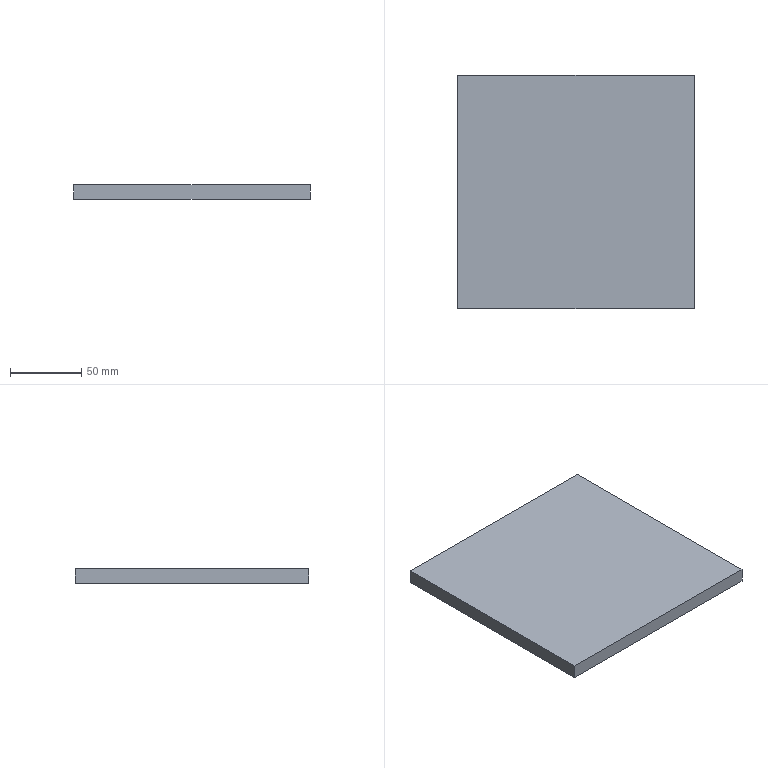Part | STEP file | 1 solid | 6 faces | box 166.259 x 164 x 10 mm | volume 272664 mm3 | plane 6
STEP:
#1=CARTESIAN_POINT('',(0.,0.,0.));
#2=DIRECTION('',(0.,0.,1.));
#3=DIRECTION('',(1.,0.,0.));
#4=AXIS2_PLACEMENT_3D('',#1,#2,#3);
#5=CARTESIAN_POINT('',(-51.848,3.164,393.641));
#6=VERTEX_POINT('',#5);
#7=CARTESIAN_POINT('',(-51.848,-160.836,393.641));
#8=VERTEX_POINT('',#7);
#9=CARTESIAN_POINT('',(-51.848,3.164,393.641));
#10=DIRECTION('',(0.,-1.,0.));
#11=VECTOR('',#10,1.);
#12=LINE('',#9,#11);
#13=CARTESIAN_POINT('',(-51.848,3.164,383.641));
#14=DIRECTION('',(-1.,0.,0.));
#15=DIRECTION('',(0.,0.,1.));
#16=AXIS2_PLACEMENT_3D('',#13,#14,#15);
#17=PLANE('',#16);
#18=CARTESIAN_POINT('',(10.,0.));
#19=DIRECTION('',(0.,-1.));
#20=VECTOR('',#19,1.);
#21=LINE('',#18,#20);
#22=(GEOMETRIC_REPRESENTATION_CONTEXT(2)PARAMETRIC_REPRESENTATION_CONTEXT()REPRESENTATION_CONTEXT('',''));
#23=DEFINITIONAL_REPRESENTATION('',(#21),#22);
#24=PCURVE('',#17,#23);
#25=CARTESIAN_POINT('',(0.,0.,393.641));
#26=DIRECTION('',(0.,0.,1.));
#27=DIRECTION('',(1.,0.,0.));
#28=AXIS2_PLACEMENT_3D('',#25,#26,#27);
#29=PLANE('',#28);
#30=CARTESIAN_POINT('',(-51.848,3.164));
#31=DIRECTION('',(0.,-1.));
#32=VECTOR('',#31,1.);
#33=LINE('',#30,#32);
#34=(GEOMETRIC_REPRESENTATION_CONTEXT(2)PARAMETRIC_REPRESENTATION_CONTEXT()REPRESENTATION_CONTEXT('',''));
#35=DEFINITIONAL_REPRESENTATION('',(#33),#34);
#36=PCURVE('',#29,#35);
#37=SURFACE_CURVE('',#12,(#24,#36),.PCURVE_S1.);
#38=EDGE_CURVE('',#6,#8,#37,.T.);
#39=ORIENTED_EDGE('',*,*,#38,.F.);
#40=CARTESIAN_POINT('',(-51.848,3.164,383.641));
#41=VERTEX_POINT('',#40);
#42=CARTESIAN_POINT('',(-51.848,3.164,383.641));
#43=DIRECTION('',(0.,0.,1.));
#44=VECTOR('',#43,1.);
#45=LINE('',#42,#44);
#46=CARTESIAN_POINT('',(0.,0.));
#47=DIRECTION('',(1.,0.));
#48=VECTOR('',#47,1.);
#49=LINE('',#46,#48);
#50=(GEOMETRIC_REPRESENTATION_CONTEXT(2)PARAMETRIC_REPRESENTATION_CONTEXT()REPRESENTATION_CONTEXT('',''));
#51=DEFINITIONAL_REPRESENTATION('',(#49),#50);
#52=PCURVE('',#17,#51);
#53=CARTESIAN_POINT('',(-51.848,3.164,383.641));
#54=DIRECTION('',(0.,1.,0.));
#55=DIRECTION('',(0.,0.,1.));
#56=AXIS2_PLACEMENT_3D('',#53,#54,#55);
#57=PLANE('',#56);
#58=CARTESIAN_POINT('',(0.,0.));
#59=DIRECTION('',(1.,0.));
#60=VECTOR('',#59,1.);
#61=LINE('',#58,#60);
#62=(GEOMETRIC_REPRESENTATION_CONTEXT(2)PARAMETRIC_REPRESENTATION_CONTEXT()REPRESENTATION_CONTEXT('',''));
#63=DEFINITIONAL_REPRESENTATION('',(#61),#62);
#64=PCURVE('',#57,#63);
#65=SURFACE_CURVE('',#45,(#52,#64),.PCURVE_S1.);
#66=EDGE_CURVE('',#41,#6,#65,.T.);
#67=ORIENTED_EDGE('',*,*,#66,.F.);
#68=CARTESIAN_POINT('',(-51.848,-160.836,383.641));
#69=VERTEX_POINT('',#68);
#70=CARTESIAN_POINT('',(-51.848,3.164,383.641));
#71=DIRECTION('',(0.,-1.,0.));
#72=VECTOR('',#71,1.);
#73=LINE('',#70,#72);
#74=CARTESIAN_POINT('',(0.,0.));
#75=DIRECTION('',(0.,-1.));
#76=VECTOR('',#75,1.);
#77=LINE('',#74,#76);
#78=(GEOMETRIC_REPRESENTATION_CONTEXT(2)PARAMETRIC_REPRESENTATION_CONTEXT()REPRESENTATION_CONTEXT('',''));
#79=DEFINITIONAL_REPRESENTATION('',(#77),#78);
#80=PCURVE('',#17,#79);
#81=CARTESIAN_POINT('',(0.,0.,383.641));
#82=DIRECTION('',(0.,0.,1.));
#83=DIRECTION('',(1.,0.,0.));
#84=AXIS2_PLACEMENT_3D('',#81,#82,#83);
#85=PLANE('',#84);
#86=CARTESIAN_POINT('',(-51.848,3.164));
#87=DIRECTION('',(0.,-1.));
#88=VECTOR('',#87,1.);
#89=LINE('',#86,#88);
#90=(GEOMETRIC_REPRESENTATION_CONTEXT(2)PARAMETRIC_REPRESENTATION_CONTEXT()REPRESENTATION_CONTEXT('',''));
#91=DEFINITIONAL_REPRESENTATION('',(#89),#90);
#92=PCURVE('',#85,#91);
#93=SURFACE_CURVE('',#73,(#80,#92),.PCURVE_S1.);
#94=EDGE_CURVE('',#41,#69,#93,.T.);
#95=ORIENTED_EDGE('',*,*,#94,.T.);
#96=CARTESIAN_POINT('',(-51.848,-160.836,383.641));
#97=DIRECTION('',(0.,0.,1.));
#98=VECTOR('',#97,1.);
#99=LINE('',#96,#98);
#100=CARTESIAN_POINT('',(0.,-164.));
#101=DIRECTION('',(1.,0.));
#102=VECTOR('',#101,1.);
#103=LINE('',#100,#102);
#104=(GEOMETRIC_REPRESENTATION_CONTEXT(2)PARAMETRIC_REPRESENTATION_CONTEXT()REPRESENTATION_CONTEXT('',''));
#105=DEFINITIONAL_REPRESENTATION('',(#103),#104);
#106=PCURVE('',#17,#105);
#107=CARTESIAN_POINT('',(-51.848,-160.836,383.641));
#108=DIRECTION('',(0.,-1.,0.));
#109=DIRECTION('',(0.,0.,-1.));
#110=AXIS2_PLACEMENT_3D('',#107,#108,#109);
#111=PLANE('',#110);
#112=CARTESIAN_POINT('',(0.,0.));
#113=DIRECTION('',(-1.,0.));
#114=VECTOR('',#113,1.);
#115=LINE('',#112,#114);
#116=(GEOMETRIC_REPRESENTATION_CONTEXT(2)PARAMETRIC_REPRESENTATION_CONTEXT()REPRESENTATION_CONTEXT('',''));
#117=DEFINITIONAL_REPRESENTATION('',(#115),#116);
#118=PCURVE('',#111,#117);
#119=SURFACE_CURVE('',#99,(#106,#118),.PCURVE_S1.);
#120=EDGE_CURVE('',#69,#8,#119,.T.);
#121=ORIENTED_EDGE('',*,*,#120,.T.);
#122=EDGE_LOOP('',(#39,#67,#95,#121));
#123=FACE_BOUND('',#122,.T.);
#124=ADVANCED_FACE('',(#123),#17,.T.);
#125=CARTESIAN_POINT('',(114.411,3.164,393.641));
#126=VERTEX_POINT('',#125);
#127=CARTESIAN_POINT('',(-51.848,3.164,393.641));
#128=DIRECTION('',(-1.,0.,0.));
#129=VECTOR('',#128,1.);
#130=LINE('',#127,#129);
#131=CARTESIAN_POINT('',(10.,0.));
#132=DIRECTION('',(0.,-1.));
#133=VECTOR('',#132,1.);
#134=LINE('',#131,#133);
#135=(GEOMETRIC_REPRESENTATION_CONTEXT(2)PARAMETRIC_REPRESENTATION_CONTEXT()REPRESENTATION_CONTEXT('',''));
#136=DEFINITIONAL_REPRESENTATION('',(#134),#135);
#137=PCURVE('',#57,#136);
#138=CARTESIAN_POINT('',(-51.848,3.164));
#139=DIRECTION('',(-1.,0.));
#140=VECTOR('',#139,1.);
#141=LINE('',#138,#140);
#142=(GEOMETRIC_REPRESENTATION_CONTEXT(2)PARAMETRIC_REPRESENTATION_CONTEXT()REPRESENTATION_CONTEXT('',''));
#143=DEFINITIONAL_REPRESENTATION('',(#141),#142);
#144=PCURVE('',#29,#143);
#145=SURFACE_CURVE('',#130,(#137,#144),.PCURVE_S1.);
#146=EDGE_CURVE('',#126,#6,#145,.T.);
#147=ORIENTED_EDGE('',*,*,#146,.F.);
#148=CARTESIAN_POINT('',(114.411,3.164,383.641));
#149=VERTEX_POINT('',#148);
#150=CARTESIAN_POINT('',(114.411,3.164,383.641));
#151=DIRECTION('',(0.,0.,1.));
#152=VECTOR('',#151,1.);
#153=LINE('',#150,#152);
#154=CARTESIAN_POINT('',(0.,166.259));
#155=DIRECTION('',(1.,0.));
#156=VECTOR('',#155,1.);
#157=LINE('',#154,#156);
#158=(GEOMETRIC_REPRESENTATION_CONTEXT(2)PARAMETRIC_REPRESENTATION_CONTEXT()REPRESENTATION_CONTEXT('',''));
#159=DEFINITIONAL_REPRESENTATION('',(#157),#158);
#160=PCURVE('',#57,#159);
#161=CARTESIAN_POINT('',(114.411,3.164,383.641));
#162=DIRECTION('',(1.,0.,0.));
#163=DIRECTION('',(0.,0.,-1.));
#164=AXIS2_PLACEMENT_3D('',#161,#162,#163);
#165=PLANE('',#164);
#166=CARTESIAN_POINT('',(0.,0.));
#167=DIRECTION('',(-1.,0.));
#168=VECTOR('',#167,1.);
#169=LINE('',#166,#168);
#170=(GEOMETRIC_REPRESENTATION_CONTEXT(2)PARAMETRIC_REPRESENTATION_CONTEXT()REPRESENTATION_CONTEXT('',''));
#171=DEFINITIONAL_REPRESENTATION('',(#169),#170);
#172=PCURVE('',#165,#171);
#173=SURFACE_CURVE('',#153,(#160,#172),.PCURVE_S1.);
#174=EDGE_CURVE('',#149,#126,#173,.T.);
#175=ORIENTED_EDGE('',*,*,#174,.F.);
#176=CARTESIAN_POINT('',(-51.848,3.164,383.641));
#177=DIRECTION('',(-1.,0.,0.));
#178=VECTOR('',#177,1.);
#179=LINE('',#176,#178);
#180=CARTESIAN_POINT('',(0.,0.));
#181=DIRECTION('',(0.,-1.));
#182=VECTOR('',#181,1.);
#183=LINE('',#180,#182);
#184=(GEOMETRIC_REPRESENTATION_CONTEXT(2)PARAMETRIC_REPRESENTATION_CONTEXT()REPRESENTATION_CONTEXT('',''));
#185=DEFINITIONAL_REPRESENTATION('',(#183),#184);
#186=PCURVE('',#57,#185);
#187=CARTESIAN_POINT('',(-51.848,3.164));
#188=DIRECTION('',(-1.,0.));
#189=VECTOR('',#188,1.);
#190=LINE('',#187,#189);
#191=(GEOMETRIC_REPRESENTATION_CONTEXT(2)PARAMETRIC_REPRESENTATION_CONTEXT()REPRESENTATION_CONTEXT('',''));
#192=DEFINITIONAL_REPRESENTATION('',(#190),#191);
#193=PCURVE('',#85,#192);
#194=SURFACE_CURVE('',#179,(#186,#193),.PCURVE_S1.);
#195=EDGE_CURVE('',#149,#41,#194,.T.);
#196=ORIENTED_EDGE('',*,*,#195,.T.);
#197=ORIENTED_EDGE('',*,*,#66,.T.);
#198=EDGE_LOOP('',(#147,#175,#196,#197));
#199=FACE_BOUND('',#198,.T.);
#200=ADVANCED_FACE('',(#199),#57,.T.);
#201=CARTESIAN_POINT('',(114.411,-160.836,393.641));
#202=VERTEX_POINT('',#201);
#203=CARTESIAN_POINT('',(114.411,3.164,393.641));
#204=DIRECTION('',(0.,1.,0.));
#205=VECTOR('',#204,1.);
#206=LINE('',#203,#205);
#207=CARTESIAN_POINT('',(-10.,0.));
#208=DIRECTION('',(0.,1.));
#209=VECTOR('',#208,1.);
#210=LINE('',#207,#209);
#211=(GEOMETRIC_REPRESENTATION_CONTEXT(2)PARAMETRIC_REPRESENTATION_CONTEXT()REPRESENTATION_CONTEXT('',''));
#212=DEFINITIONAL_REPRESENTATION('',(#210),#211);
#213=PCURVE('',#165,#212);
#214=CARTESIAN_POINT('',(114.411,3.164));
#215=DIRECTION('',(0.,1.));
#216=VECTOR('',#215,1.);
#217=LINE('',#214,#216);
#218=(GEOMETRIC_REPRESENTATION_CONTEXT(2)PARAMETRIC_REPRESENTATION_CONTEXT()REPRESENTATION_CONTEXT('',''));
#219=DEFINITIONAL_REPRESENTATION('',(#217),#218);
#220=PCURVE('',#29,#219);
#221=SURFACE_CURVE('',#206,(#213,#220),.PCURVE_S1.);
#222=EDGE_CURVE('',#202,#126,#221,.T.);
#223=ORIENTED_EDGE('',*,*,#222,.F.);
#224=CARTESIAN_POINT('',(114.411,-160.836,383.641));
#225=VERTEX_POINT('',#224);
#226=CARTESIAN_POINT('',(114.411,-160.836,383.641));
#227=DIRECTION('',(0.,0.,1.));
#228=VECTOR('',#227,1.);
#229=LINE('',#226,#228);
#230=CARTESIAN_POINT('',(0.,-164.));
#231=DIRECTION('',(-1.,0.));
#232=VECTOR('',#231,1.);
#233=LINE('',#230,#232);
#234=(GEOMETRIC_REPRESENTATION_CONTEXT(2)PARAMETRIC_REPRESENTATION_CONTEXT()REPRESENTATION_CONTEXT('',''));
#235=DEFINITIONAL_REPRESENTATION('',(#233),#234);
#236=PCURVE('',#165,#235);
#237=CARTESIAN_POINT('',(0.,166.259));
#238=DIRECTION('',(-1.,0.));
#239=VECTOR('',#238,1.);
#240=LINE('',#237,#239);
#241=(GEOMETRIC_REPRESENTATION_CONTEXT(2)PARAMETRIC_REPRESENTATION_CONTEXT()REPRESENTATION_CONTEXT('',''));
#242=DEFINITIONAL_REPRESENTATION('',(#240),#241);
#243=PCURVE('',#111,#242);
#244=SURFACE_CURVE('',#229,(#236,#243),.PCURVE_S1.);
#245=EDGE_CURVE('',#225,#202,#244,.T.);
#246=ORIENTED_EDGE('',*,*,#245,.F.);
#247=CARTESIAN_POINT('',(114.411,3.164,383.641));
#248=DIRECTION('',(0.,1.,0.));
#249=VECTOR('',#248,1.);
#250=LINE('',#247,#249);
#251=CARTESIAN_POINT('',(0.,0.));
#252=DIRECTION('',(0.,1.));
#253=VECTOR('',#252,1.);
#254=LINE('',#251,#253);
#255=(GEOMETRIC_REPRESENTATION_CONTEXT(2)PARAMETRIC_REPRESENTATION_CONTEXT()REPRESENTATION_CONTEXT('',''));
#256=DEFINITIONAL_REPRESENTATION('',(#254),#255);
#257=PCURVE('',#165,#256);
#258=CARTESIAN_POINT('',(114.411,3.164));
#259=DIRECTION('',(0.,1.));
#260=VECTOR('',#259,1.);
#261=LINE('',#258,#260);
#262=(GEOMETRIC_REPRESENTATION_CONTEXT(2)PARAMETRIC_REPRESENTATION_CONTEXT()REPRESENTATION_CONTEXT('',''));
#263=DEFINITIONAL_REPRESENTATION('',(#261),#262);
#264=PCURVE('',#85,#263);
#265=SURFACE_CURVE('',#250,(#257,#264),.PCURVE_S1.);
#266=EDGE_CURVE('',#225,#149,#265,.T.);
#267=ORIENTED_EDGE('',*,*,#266,.T.);
#268=ORIENTED_EDGE('',*,*,#174,.T.);
#269=EDGE_LOOP('',(#223,#246,#267,#268));
#270=FACE_BOUND('',#269,.T.);
#271=ADVANCED_FACE('',(#270),#165,.T.);
#272=CARTESIAN_POINT('',(-51.848,-160.836,393.641));
#273=DIRECTION('',(1.,0.,0.));
#274=VECTOR('',#273,1.);
#275=LINE('',#272,#274);
#276=CARTESIAN_POINT('',(-10.,0.));
#277=DIRECTION('',(0.,1.));
#278=VECTOR('',#277,1.);
#279=LINE('',#276,#278);
#280=(GEOMETRIC_REPRESENTATION_CONTEXT(2)PARAMETRIC_REPRESENTATION_CONTEXT()REPRESENTATION_CONTEXT('',''));
#281=DEFINITIONAL_REPRESENTATION('',(#279),#280);
#282=PCURVE('',#111,#281);
#283=CARTESIAN_POINT('',(-51.848,-160.836));
#284=DIRECTION('',(1.,0.));
#285=VECTOR('',#284,1.);
#286=LINE('',#283,#285);
#287=(GEOMETRIC_REPRESENTATION_CONTEXT(2)PARAMETRIC_REPRESENTATION_CONTEXT()REPRESENTATION_CONTEXT('',''));
#288=DEFINITIONAL_REPRESENTATION('',(#286),#287);
#289=PCURVE('',#29,#288);
#290=SURFACE_CURVE('',#275,(#282,#289),.PCURVE_S1.);
#291=EDGE_CURVE('',#8,#202,#290,.T.);
#292=ORIENTED_EDGE('',*,*,#291,.F.);
#293=ORIENTED_EDGE('',*,*,#120,.F.);
#294=CARTESIAN_POINT('',(-51.848,-160.836,383.641));
#295=DIRECTION('',(1.,0.,0.));
#296=VECTOR('',#295,1.);
#297=LINE('',#294,#296);
#298=CARTESIAN_POINT('',(0.,0.));
#299=DIRECTION('',(0.,1.));
#300=VECTOR('',#299,1.);
#301=LINE('',#298,#300);
#302=(GEOMETRIC_REPRESENTATION_CONTEXT(2)PARAMETRIC_REPRESENTATION_CONTEXT()REPRESENTATION_CONTEXT('',''));
#303=DEFINITIONAL_REPRESENTATION('',(#301),#302);
#304=PCURVE('',#111,#303);
#305=CARTESIAN_POINT('',(-51.848,-160.836));
#306=DIRECTION('',(1.,0.));
#307=VECTOR('',#306,1.);
#308=LINE('',#305,#307);
#309=(GEOMETRIC_REPRESENTATION_CONTEXT(2)PARAMETRIC_REPRESENTATION_CONTEXT()REPRESENTATION_CONTEXT('',''));
#310=DEFINITIONAL_REPRESENTATION('',(#308),#309);
#311=PCURVE('',#85,#310);
#312=SURFACE_CURVE('',#297,(#304,#311),.PCURVE_S1.);
#313=EDGE_CURVE('',#69,#225,#312,.T.);
#314=ORIENTED_EDGE('',*,*,#313,.T.);
#315=ORIENTED_EDGE('',*,*,#245,.T.);
#316=EDGE_LOOP('',(#292,#293,#314,#315));
#317=FACE_BOUND('',#316,.T.);
#318=ADVANCED_FACE('',(#317),#111,.T.);
#319=ORIENTED_EDGE('',*,*,#94,.F.);
#320=ORIENTED_EDGE('',*,*,#195,.F.);
#321=ORIENTED_EDGE('',*,*,#266,.F.);
#322=ORIENTED_EDGE('',*,*,#313,.F.);
#323=EDGE_LOOP('',(#319,#320,#321,#322));
#324=FACE_BOUND('',#323,.T.);
#325=ADVANCED_FACE('',(#324),#85,.F.);
#326=ORIENTED_EDGE('',*,*,#38,.T.);
#327=ORIENTED_EDGE('',*,*,#291,.T.);
#328=ORIENTED_EDGE('',*,*,#222,.T.);
#329=ORIENTED_EDGE('',*,*,#146,.T.);
#330=EDGE_LOOP('',(#326,#327,#328,#329));
#331=FACE_BOUND('',#330,.T.);
#332=ADVANCED_FACE('',(#331),#29,.T.);
#333=CLOSED_SHELL('',(#124,#200,#271,#318,#325,#332));
#334=MANIFOLD_SOLID_BREP('',#333);
#335=(LENGTH_UNIT()NAMED_UNIT(*)SI_UNIT(.MILLI.,.METRE.));
#336=UNCERTAINTY_MEASURE_WITH_UNIT(LENGTH_MEASURE(0.0000001),#335,'','');
#337=(NAMED_UNIT(*)PLANE_ANGLE_UNIT()SI_UNIT($,.RADIAN.));
#338=(NAMED_UNIT(*)SI_UNIT($,.STERADIAN.)SOLID_ANGLE_UNIT());
#339=(GEOMETRIC_REPRESENTATION_CONTEXT(3)GLOBAL_UNCERTAINTY_ASSIGNED_CONTEXT((#336))GLOBAL_UNIT_ASSIGNED_CONTEXT((#335,#337,#338))REPRESENTATION_CONTEXT('',''));
#340=ADVANCED_BREP_SHAPE_REPRESENTATION('',(#4,#334),#339);